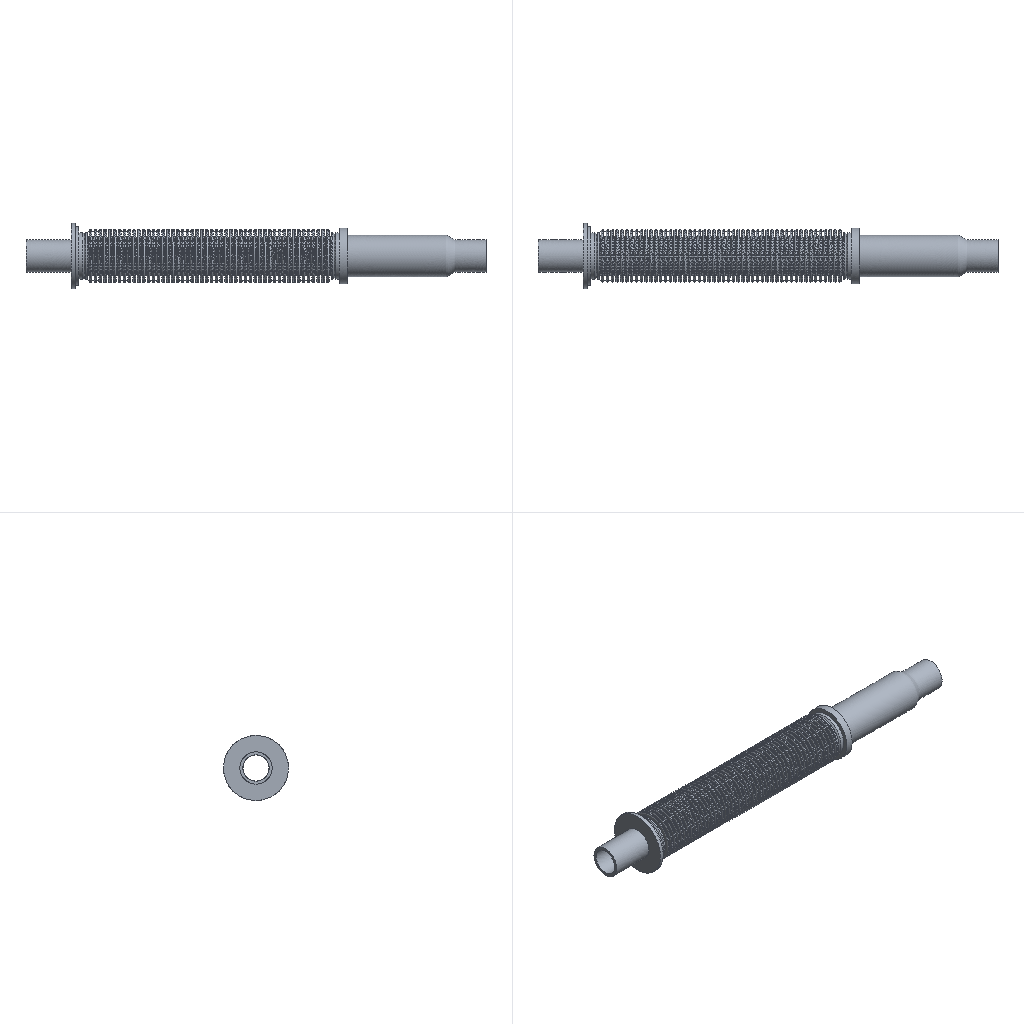Simulation study | ansys workbench
Set-up summary:
category,name,step,type,value,unit,region
solver,ansys_workbench
units,mm-N-s-tonne (MPa),,stated,"/units,MPA"
analysis,LS1,,static
load_step,LS1,LS1,static,nsubst=1; time=1
mesh,nodes,,,678968
mesh,elements,,,370861
element_type,SOLID187,,,351223
element_type,SURF154,,,16496
element_type,TARGE170,,,1571
element_type,CONTA174,,,1571
material,316l,,E,190000,tonne s^-2 mm^-1
material,316l,,nu,0.3
material,316l,,density,7.98e-09,tonne mm^-3
material,316l,,conductivity,60.5,tonne mm s^-3 C^-1
material,316l,,specific_heat,4.34e+08,mm^2 s^-2 C^-1
material,316l,,cte,1.3e-05,C^-1
material,316l,,permeability,10000
material,316l,,resistivity,0.00017,ohm mm
load,"Define Pressure Using Surface Effect Elements ""__""",LS1,pressure,3,,SURF154 #8
load,Component For All Non-Zero UX Displacements,LS1,body load temp,-296,,_CM43
bc,Fixed Supports,model,fixed,[dofs=ALL],,_FIXEDSU
bc,Set Displacements,LS1,prescribed ux,-50 [dofs=UX],,_CM49UX_XP
contact,Contact Region,,bonded (always),element=CONTA174
contact,Contact Region 2,,bonded (always),element=CONTA174
named_set,_FIXEDSU,,node,976
named_set,_CM49UX_XP,,node,372
Ansys APDL input file, long lists of numbers shortened:
/batch
/config,noeldb,1     ! force off writing results to database
*get,_wallstrt,active,,time,wall
! ANSYS input file written by Workbench version 2022 R1
! File used for geometry attach:
/title,wbnew--____ (B5)
! ****** Begin Custom Load Command Snippet ******
/COM, ACT Extensions:
/COM,     LSDYNA, 2021.1
/COM,
! ****** End   Custom Load Command Snippet ******
*DIM,_wb_ProjectScratch_dir,string,248
_wb_ProjectScratch_dir(1) = ''
*DIM,_wb_SolverFiles_dir,string,248
_wb_SolverFiles_dir(1) = ''
*DIM,_wb_userfiles_dir,string,248
_wb_userfiles_dir(1) = ''
/com,--- Data in consistent NMM units. See Solving Units in the help system for more information.
/units,MPA
/nopr
/wb,file,start              !  signify a WB generated input file
/prep7
! Turn off shape checking because checks already performed inside WB mesher.
! See help system for more information.
SHPP,OFF,,NOWARN
/nolist
etcon,set             ! allow ANSYS to choose best KEYOP's for 180x elements, resets any applicable keyopt to MAPDL defaults
/com,*********** Nodes for the whole assembly ***********
nblock,3,,746864
(1i9,3e20.9e3)
        1    -2.384542767E+01     4.925080413E+01     7.465016973E+01
! (678967 more lines like these left out)
-1
/wb,elem,start            !  set before creation of elements
/com,*********** Elements for Body 1 "-01__1______|__1" ***********
et,1,187
eblock,19,solid,,26262
(19i9)
        1        1        1        1        0        0        0        0       10        0        1     6275     7134     7442     7293    43482    46775    43491    43488
! (52523 more lines like these left out)
-1
/com,*********** Elements for Body 2 "-02___|__1" ***********
et,2,187
eblock,19,solid,,257584
(19i9)
        2        2        2        2        0        0        0        0       10        0    93640   169172   187383   235598   235585   265563   397741   265566   265565
! (515167 more lines like these left out)
-1
/com,*********** Elements for Body 3 "-05__2|__1" ***********
et,3,187
eblock,19,solid,,67377
(19i9)
        3        3        3        3        0        0        0        0       10        0    26263    62283    65957    65826    65947   157086   167429   157083   157085
! (134753 more lines like these left out)
-1
/wb,elem,end               !  done creating elements
/com,*********** Send User Defined Coordinate System(s) ***********
csys,0
toffst,273.15,  ! Temperature offset from absolute zero
/com,*********** Set Reference Temperature ***********
tref,22.
/wb,mat,start              !  starting to send materials
/com,*********** Send Materials ***********
Temperature = 'TEMP' ! Temperature
MP,DENS,1,7.98e-09,	! tonne mm^-3
MP,ALPX,1,1.3e-05,	! C^-1
MP,C,1,434000000,	! mm^2 s^-2 C^-1
MP,KXX,1,60.5,	! tonne mm s^-3 C^-1
MP,RSVX,1,0.00017,	! ohm mm
MP,EX,1,190000,	! tonne s^-2 mm^-1
MP,NUXY,1,0.3,
MP,MURX,1,10000,
Temperature = 'TEMP' ! Temperature
MP,DENS,2,7.98e-09,	! tonne mm^-3
MP,ALPX,2,1.3e-05,	! C^-1
MP,C,2,434000000,	! mm^2 s^-2 C^-1
MP,KXX,2,60.5,	! tonne mm s^-3 C^-1
MP,RSVX,2,0.00017,	! ohm mm
MP,EX,2,190000,	! tonne s^-2 mm^-1
MP,NUXY,2,0.3,
MP,MURX,2,10000,
Temperature = 'TEMP' ! Temperature
MP,DENS,3,7.98e-09,	! tonne mm^-3
MP,ALPX,3,1.3e-05,	! C^-1
MP,C,3,434000000,	! mm^2 s^-2 C^-1
MP,KXX,3,60.5,	! tonne mm s^-3 C^-1
MP,RSVX,3,0.00017,	! ohm mm
MP,EX,3,190000,	! tonne s^-2 mm^-1
MP,NUXY,3,0.3,
MP,MURX,3,10000,
/wb,mat,end                !  done sending materials
!************************* Model Summary ********************
!-01__1______|__1,	316l,	matid,	1
!-02___|__1,	316l,	matid,	2
!-05__2|__1,	316l,	matid,	3
!************************* End Model Summary ********************
! get the diagonal of the bounding box. Needed later for other things
*get,_xmin,node,,mnloc,x
*get,_ymin,node,,mnloc,y
*get,_zmin,node,,mnloc,z
*get,_xmax,node,,mxloc,x
*get,_ymax,node,,mxloc,y
*get,_zmax,node,,mxloc,z
_ASMDIAG=(_xmax-_xmin)*(_xmax-_xmin)+(_ymax-_ymin)*(_ymax-_ymin)+(_zmax-_zmin)*(_zmax-_zmin)
_ASMDIAG=SQRT(_ASMDIAG)
/wb,contact,start          !  starting to send contact
/com,*********** Create Contact "接触区域" ***********
/com,            Real Constant Set For Above Contact Is 5 & 4
*set,tid,5
*set,cid,4
r,tid
r,cid
et,tid,170
et,cid,174
eblock,10,,,413
(15i9)
   562074        5        5        5        0     5347     5437     5386     5386    38609    38881     5386    38607
! (412 more lines like these left out)
-1
eblock,10,,,413
(15i9)
   562487        4        4        4        0     5347     5437     5386     5386    38609    38881     5386    38607
! (412 more lines like these left out)
-1
eblock,10,,,445
(15i9)
   562900        4        5        4        0   175882   175883   240659   240659   317758   317773   240659   317764
! (444 more lines like these left out)
-1
eblock,10,,,445
(15i9)
   563345        5        4        5        0   175882   175883   240659   240659   317758   317773   240659   317764
! (444 more lines like these left out)
-1
keyo,cid,8,2               ! auto create asymmetric contact (from Program Controlled setting)
keyo,cid,10,0              ! adjust contact stiffness each NR iteration (from Program Controlled setting)
keyo,cid,12,5              ! bonded always
keyo,cid,18,1              ! small sliding turned on by application
keyo,cid,2,0               ! augmented Lagrange (from Program Controlled setting)
keyo,cid,4,0               ! on Gauss point (from Program Controlled setting)
keyo,cid,9,1               ! ignore initial gaps/penetration
keyo,cid,7,0               ! No Prediction
rmod,tid,3,10.      ! FKN
rmod,tid,5,0.       ! ICONT
rmod,tid,6,0.       ! PINB
rmod,tid,10,0.      ! CNOF
rmod,tid,12,0.      ! FKT
rmod,tid,36,32      ! WB DSID
rmod,cid,3,10.      ! FKN
rmod,cid,5,0.       ! ICONT
rmod,cid,6,0.       ! PINB
rmod,cid,10,0.      ! CNOF
rmod,cid,12,0.      ! FKT
rmod,cid,36,32      ! WB DSID
/com,*********** Create Contact "接触区域 2" ***********
/com,            Real Constant Set For Above Contact Is 7 & 6
*set,tid,7
*set,cid,6
r,tid
r,cid
et,tid,170
et,cid,174
eblock,10,,,445
(15i9)
   563790        7        7        7        0   174051   241111   174050   174050   303475   303466   174050   303458
! (444 more lines like these left out)
-1
eblock,10,,,445
(15i9)
   564235        6        6        6        0   174051   241111   174050   174050   303475   303466   174050   303458
! (444 more lines like these left out)
-1
eblock,10,,,268
(15i9)
   564680        6        7        6        0    48303    61995    48304    48304    75358    75362    48304    75355
! (267 more lines like these left out)
-1
eblock,10,,,268
(15i9)
   564948        7        6        7        0    48303    61995    48304    48304    75358    75362    48304    75355
! (267 more lines like these left out)
-1
keyo,cid,8,2               ! auto create asymmetric contact (from Program Controlled setting)
keyo,cid,10,0              ! adjust contact stiffness each NR iteration (from Program Controlled setting)
keyo,cid,12,5              ! bonded always
keyo,cid,18,1              ! small sliding turned on by application
keyo,cid,2,0               ! augmented Lagrange (from Program Controlled setting)
keyo,cid,4,0               ! on Gauss point (from Program Controlled setting)
keyo,cid,9,1               ! ignore initial gaps/penetration
keyo,cid,7,0               ! No Prediction
rmod,tid,3,10.      ! FKN
rmod,tid,5,0.       ! ICONT
rmod,tid,6,0.       ! PINB
rmod,tid,10,0.      ! CNOF
rmod,tid,12,0.      ! FKT
rmod,tid,36,35      ! WB DSID
rmod,cid,3,10.      ! FKN
rmod,cid,5,0.       ! ICONT
rmod,cid,6,0.       ! PINB
rmod,cid,10,0.      ! CNOF
rmod,cid,12,0.      ! FKT
rmod,cid,36,35      ! WB DSID
nsel,all
esel,all
/wb,contact,end            !  done creating contacts
/golist
/wb,load,start             !  starting to send loads
/com,*********** Fixed Supports ***********
CMBLOCK,_FIXEDSU,NODE,      976
(8i10)
         1         2         3         4         5         6         7         8
! (121 more lines like these left out)
cmsel,s,_FIXEDSU
d,all,all
nsel,all
/com,*********** Define Pressure Using Surface Effect Elements "__" ***********
et,8,154
eblock,10,,,16496
(15i9)
   565216        8        8        8        0    47932    47931    52673    52673    72743    72746    52673    72753
! (16495 more lines like these left out)
-1
esel,s,type,,8
keyop,8,7,0                ! Use deformed area for application of load
esel,all
/com,*********** Define Body Force Temperature ***********
esel,none
esel,a,type,,1
esel,a,type,,2,3
cm,_CM43,elem
esel,all
esel,all
/gst,on,on
fini
*get,_numnode,node,0,count
*get,_numelem,elem,0,count
*get, _MAXELEMNUM, elem, 0, NUM, MAX
*get, _MAXNODENUM, node, 0, NUM, MAX
*get, _MAXELEMTYPE, etyp, 0, NUM, MAX
*get, _MAXREALCONST, real, 0, NUM, MAX
/go
/wb,load,end               !  done creating loads
/com,--- Number of total nodes = %_numnode%
/com,--- Number of contact elements = 19638
/com,--- Number of spring elements = 0
/com,--- Number of bearing elements = 0
/com,--- Number of solid elements = 351223
/com,--- Number of condensed parts = 0
/com,--- Number of total elements = %_numelem%
*get,_wallbsol,active,,time,wall
/com,****************************************************************************
/com,*************************    SOLUTION       ********************************
/com,****************************************************************************
/solu
antype,0                   ! static analysis
_thickRatio=0.667   ! Ratio of thick parts in the model
eqsl,pcg,1e-8,,,,,,1
cntr,print,1               ! print out contact info and also make no initial contact an error
dmpoption,emat,no             ! Don't combine emat file for DANSYS
dmpoption,esav,no             ! Don't combine esav file for DANSYS
nldiag,cont,iter           ! print out contact info each equilibrium iteration
rescontrol,,none                 ! Do not keep any restart files
/com,****************************************************
/com,******************* SOLVE FOR LS 1 OF 1 ****************
esel,s,type,,8
nsle
sf,all,pres,3.
nsel,all
esel,all
/com,*** Set Displacements ***
CMBLOCK,_CM49UX_XP,NODE,      372
(8i10)
     47738     47759     47760     47761     47762     47763     47764     47765
! (46 more lines like these left out)
cmsel,s,_CM49UX_XP
d,all,ux,-50.
nsel,all
/com,*** Component For All Non-Zero UX Displacements ***
cmsel,s,_CM49ux_xp
cm,_DISPNONZEROUX,NODE
nsel,all
esel,all
/nopr
cmsel,s,_CM43
nsle
bf,all,temp,-296.
nsel,all
esel,all
/gopr
nsub,1,1,1
time,1.
outres,erase
outres,all,none
outres,nsol,all,
outres,rsol,all
outres,eangl,all
outres,etmp,all
outres,veng,all
outres,strs,all,
outres,epel,all,
outres,eppl,all,
outres,epth,all,
outres,cont,all,
! *********** WB SOLVE COMMAND ***********
! check interactive state
*get,ANSINTER_,active,,int
*if,ANSINTER_,ne,0,then
/eof
*endif
solve
/com *************** Write FE CONNECTORS *********
CEWRITE,file,ce,,INTE
/com,****************************************************
/com,*************** FINISHED SOLVE FOR LS 1 *************
*get,_wallasol,active,,time,wall
/nopr
*get,_numnode,node,0,count
*get,_numelem,elem,0,count
*get, _MAXELEMNUM, elem, 0, NUM, MAX
*get, _MAXNODENUM, node, 0, NUM, MAX,,,INTERNAL
*get, _MAXELEMTYPE, etyp, 0, NUM, MAX
*get, _MAXREALCONST, real, 0, NUM, MAX
/gopr
*get,_PCGITER,active,,solu,cgiter
/post1
xmlo,ENCODING,ISO-8859-1
xmlo,parm
/xml,parm,xml
fini
/gopr
*get,_walldone,active,,time,wall
_preptime=(_wallbsol-_wallstrt)*3600
_solvtime=(_wallasol-_wallbsol)*3600
_posttime=(_walldone-_wallasol)*3600
_totaltim=(_walldone-_wallstrt)*3600
*get,_dlbratio,active,0,solu,dlbr
*get,_combtime,active,0,solu,comb
*get,_ssmode,active,0,solu,ssmm
*get,_ndofs,active,0,solu,ndof
*get,_sol_end_time,active,0,set,time
*if,_sol_end_time,eq,1.,then
/fclean				!clean distributed files
*endif
/com,--- Total number of nodes = %_numnode%
/com,--- Total number of elements = %_numelem%
/com,--- Element load balance ratio = %_dlbratio%
/com,--- Time to combine distributed files = %_combtime%
/com,--- Sparse memory mode = %_ssmode%
/com,--- Number of DOF = %_ndofs%
/wb,file,end               ! done with WB generated input
Results summary:
result,analyses[0].index,,,1
result,analyses[0].system,,,SYS
result,analyses[0].deck,,,deck.dat
result,analyses[0].solve_status,,,completed
result,analyses[0].analysis_type,,,static
result,analyses[0].physics,,,mechanical
result,analyses[0].unit_system,,,"NMM: mm, ton, N, s, mV, mA, degC"
result,analyses[0].n_sets,,,1
result,analyses[0].load_steps[0].set,set=1,,1
result,analyses[0].load_steps[0].time_or_freq,set=1,,1
result,analyses[0].load_steps[0].max_displacement_magnitude,set=1,,50
result,analyses[0].load_steps[0].max_von_mises_nodal,set=1,,7089.4
result,analyses[0].load_steps[0].reaction_force_sum_xyz[1],set=1,,-0.1769
result,analyses[0].load_steps[0].reaction_force_sum_xyz[2],set=1,,0.01731
result,analyses[0].load_steps[0].reaction_force_sum_xyz[3],set=1,,-0.03007